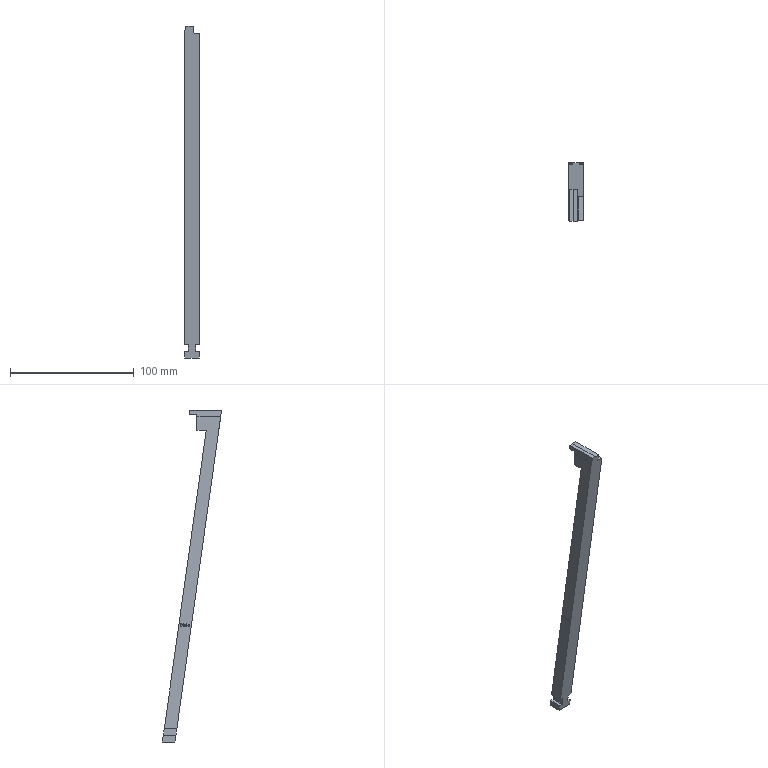Part | Creo | 1 solid | 112 faces | box 12 x 47.744 x 267.86 mm | volume 33343 mm3 | plane 54 | other 51 | cylinder 7 | commonest cylinder face diameters 1 x4 1.594 x1 2 x1 25.135 x1